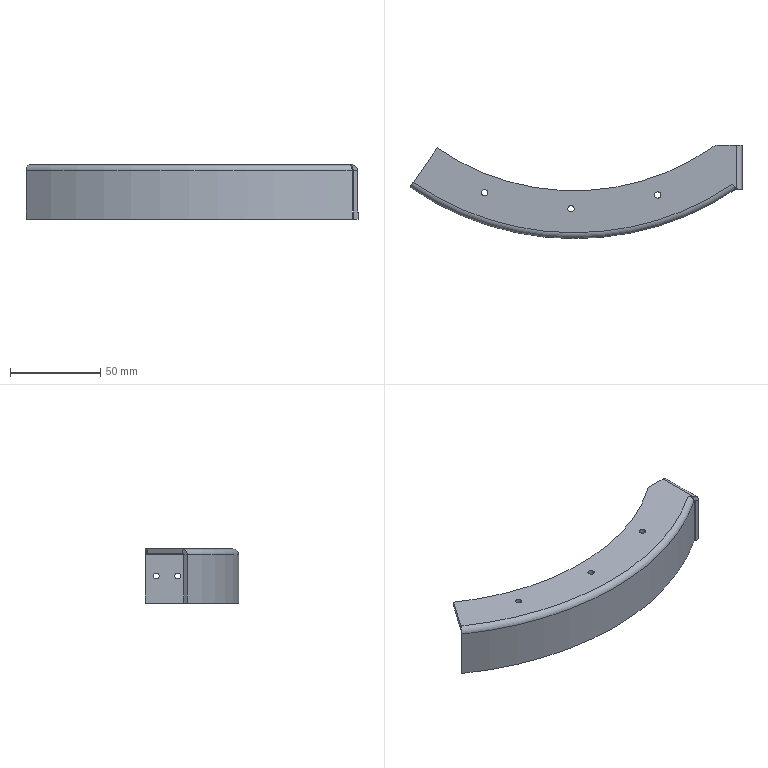Part | SolidWorks | features EdgeFlange 2, 3DProfileFeature 1, Cut 1, Fillet 1, FlatPattern 1, HoleWzd 1, ICE 1, SMBaseFlange 1, SheetMetal 1 | 1 solid | 35 faces | box 184.199 x 51.718 x 30 mm | volume 26604 mm3 | cylinder 16 | plane 16 | torus 2 | spline 1 | commonest cylinder face diameters 3.5 x6 3.3 x4 1.473 x1 6.473 x1 10 x1 267 x1
STEP:
#1=CARTESIAN_POINT('',(90.553,-126.282,-13.35));
#2=VERTEX_POINT('',#1);
#3=CARTESIAN_POINT('',(90.553,-126.282,-16.65));
#4=VERTEX_POINT('',#3);
#5=CARTESIAN_POINT('',(90.553,-126.282,-15.));
#6=DIRECTION('',(1.,0.,0.));
#7=DIRECTION('',(0.,0.,-1.));
#8=AXIS2_PLACEMENT_3D('',#5,#6,#7);
#9=CIRCLE('',#8,1.65);
#10=EDGE_CURVE('',#2,#4,#9,.T.);
#11=ORIENTED_EDGE('',*,*,#10,.F.);
#12=CARTESIAN_POINT('',(93.053,-126.282,-13.35));
#13=VERTEX_POINT('',#12);
#14=CARTESIAN_POINT('',(93.053,-126.282,-13.35));
#15=DIRECTION('',(1.,0.,0.));
#16=VECTOR('',#15,1000.);
#17=LINE('',#14,#16);
#18=EDGE_CURVE('',#2,#13,#17,.T.);
#19=ORIENTED_EDGE('',*,*,#18,.T.);
#20=CARTESIAN_POINT('',(93.053,-126.282,-16.65));
#21=VERTEX_POINT('',#20);
#22=CARTESIAN_POINT('',(93.053,-126.282,-15.));
#23=DIRECTION('',(1.,0.,0.));
#24=DIRECTION('',(0.,0.,-1.));
#25=AXIS2_PLACEMENT_3D('',#22,#23,#24);
#26=CIRCLE('',#25,1.65);
#27=EDGE_CURVE('',#13,#21,#26,.T.);
#28=ORIENTED_EDGE('',*,*,#27,.T.);
#29=CARTESIAN_POINT('',(93.053,-126.282,-16.65));
#30=DIRECTION('',(1.,0.,0.));
#31=VECTOR('',#30,1000.);
#32=LINE('',#29,#31);
#33=EDGE_CURVE('',#4,#21,#32,.T.);
#34=ORIENTED_EDGE('',*,*,#33,.F.);
#35=EDGE_LOOP('',(#11,#19,#28,#34));
#36=FACE_OUTER_BOUND('',#35,.T.);
#37=CARTESIAN_POINT('',(93.053,-126.282,-15.));
#38=DIRECTION('',(1.,0.,0.));
#39=DIRECTION('',(0.,0.,-1.));
#40=AXIS2_PLACEMENT_3D('',#37,#38,#39);
#41=CYLINDRICAL_SURFACE('',#40,1.65);
#42=ADVANCED_FACE('',(#36),#41,.F.);
#43=CARTESIAN_POINT('',(90.553,-114.282,-13.35));
#44=VERTEX_POINT('',#43);
#45=CARTESIAN_POINT('',(90.553,-114.282,-16.65));
#46=VERTEX_POINT('',#45);
#47=CARTESIAN_POINT('',(90.553,-114.282,-15.));
#48=DIRECTION('',(1.,0.,0.));
#49=DIRECTION('',(0.,0.,-1.));
#50=AXIS2_PLACEMENT_3D('',#47,#48,#49);
#51=CIRCLE('',#50,1.65);
#52=EDGE_CURVE('',#44,#46,#51,.T.);
#53=ORIENTED_EDGE('',*,*,#52,.F.);
#54=CARTESIAN_POINT('',(93.053,-114.282,-13.35));
#55=VERTEX_POINT('',#54);
#56=CARTESIAN_POINT('',(93.053,-114.282,-13.35));
#57=DIRECTION('',(1.,0.,0.));
#58=VECTOR('',#57,1000.);
#59=LINE('',#56,#58);
#60=EDGE_CURVE('',#44,#55,#59,.T.);
#61=ORIENTED_EDGE('',*,*,#60,.T.);
#62=CARTESIAN_POINT('',(93.053,-114.282,-16.65));
#63=VERTEX_POINT('',#62);
#64=CARTESIAN_POINT('',(93.053,-114.282,-15.));
#65=DIRECTION('',(1.,0.,0.));
#66=DIRECTION('',(0.,0.,-1.));
#67=AXIS2_PLACEMENT_3D('',#64,#65,#66);
#68=CIRCLE('',#67,1.65);
#69=EDGE_CURVE('',#55,#63,#68,.T.);
#70=ORIENTED_EDGE('',*,*,#69,.T.);
#71=CARTESIAN_POINT('',(93.053,-114.282,-16.65));
#72=DIRECTION('',(1.,0.,0.));
#73=VECTOR('',#72,1000.);
#74=LINE('',#71,#73);
#75=EDGE_CURVE('',#46,#63,#74,.T.);
#76=ORIENTED_EDGE('',*,*,#75,.F.);
#77=EDGE_LOOP('',(#53,#61,#70,#76));
#78=FACE_OUTER_BOUND('',#77,.T.);
#79=CARTESIAN_POINT('',(93.053,-114.282,-15.));
#80=DIRECTION('',(1.,0.,0.));
#81=DIRECTION('',(0.,0.,-1.));
#82=AXIS2_PLACEMENT_3D('',#79,#80,#81);
#83=CYLINDRICAL_SURFACE('',#82,1.65);
#84=ADVANCED_FACE('',(#78),#83,.F.);
#85=CARTESIAN_POINT('',(-3.57,-143.488,-2.5));
#86=VERTEX_POINT('',#85);
#87=CARTESIAN_POINT('',(-0.07006,-143.488,-2.5));
#88=VERTEX_POINT('',#87);
#89=CARTESIAN_POINT('',(-1.82,-143.488,-2.5));
#90=DIRECTION('',(0.,0.,1.));
#91=DIRECTION('',(1.,0.,0.));
#92=AXIS2_PLACEMENT_3D('',#89,#90,#91);
#93=CIRCLE('',#92,1.75);
#94=EDGE_CURVE('',#86,#88,#93,.T.);
#95=ORIENTED_EDGE('',*,*,#94,.F.);
#96=CARTESIAN_POINT('',(-3.57,-143.488,0.));
#97=VERTEX_POINT('',#96);
#98=CARTESIAN_POINT('',(-3.57,-143.488,-30.));
#99=DIRECTION('',(0.,0.,1.));
#100=VECTOR('',#99,1000.);
#101=LINE('',#98,#100);
#102=EDGE_CURVE('',#86,#97,#101,.T.);
#103=ORIENTED_EDGE('',*,*,#102,.T.);
#104=CARTESIAN_POINT('',(-0.07006,-143.488,0.));
#105=VERTEX_POINT('',#104);
#106=CARTESIAN_POINT('',(-1.82,-143.488,0.));
#107=DIRECTION('',(0.,0.,1.));
#108=DIRECTION('',(1.,0.,0.));
#109=AXIS2_PLACEMENT_3D('',#106,#107,#108);
#110=CIRCLE('',#109,1.75);
#111=EDGE_CURVE('',#97,#105,#110,.T.);
#112=ORIENTED_EDGE('',*,*,#111,.T.);
#113=CARTESIAN_POINT('',(-0.07006,-143.488,-30.));
#114=DIRECTION('',(0.,0.,1.));
#115=VECTOR('',#114,1000.);
#116=LINE('',#113,#115);
#117=EDGE_CURVE('',#88,#105,#116,.T.);
#118=ORIENTED_EDGE('',*,*,#117,.F.);
#119=EDGE_LOOP('',(#95,#103,#112,#118));
#120=FACE_OUTER_BOUND('',#119,.T.);
#121=CARTESIAN_POINT('',(-1.82,-143.488,-30.));
#122=DIRECTION('',(0.,0.,1.));
#123=DIRECTION('',(1.,0.,0.));
#124=AXIS2_PLACEMENT_3D('',#121,#122,#123);
#125=CYLINDRICAL_SURFACE('',#124,1.75);
#126=ADVANCED_FACE('',(#120),#125,.F.);
#127=CARTESIAN_POINT('',(44.55,-135.825,-2.5));
#128=VERTEX_POINT('',#127);
#129=CARTESIAN_POINT('',(48.05,-135.825,-2.5));
#130=VERTEX_POINT('',#129);
#131=CARTESIAN_POINT('',(46.3,-135.825,-2.5));
#132=DIRECTION('',(0.,0.,1.));
#133=DIRECTION('',(1.,0.,0.));
#134=AXIS2_PLACEMENT_3D('',#131,#132,#133);
#135=CIRCLE('',#134,1.75);
#136=EDGE_CURVE('',#128,#130,#135,.T.);
#137=ORIENTED_EDGE('',*,*,#136,.F.);
#138=CARTESIAN_POINT('',(44.55,-135.825,0.));
#139=VERTEX_POINT('',#138);
#140=CARTESIAN_POINT('',(44.55,-135.825,-30.));
#141=DIRECTION('',(0.,0.,1.));
#142=VECTOR('',#141,1000.);
#143=LINE('',#140,#142);
#144=EDGE_CURVE('',#128,#139,#143,.T.);
#145=ORIENTED_EDGE('',*,*,#144,.T.);
#146=CARTESIAN_POINT('',(48.05,-135.825,0.));
#147=VERTEX_POINT('',#146);
#148=CARTESIAN_POINT('',(46.3,-135.825,0.));
#149=DIRECTION('',(0.,0.,1.));
#150=DIRECTION('',(1.,0.,0.));
#151=AXIS2_PLACEMENT_3D('',#148,#149,#150);
#152=CIRCLE('',#151,1.75);
#153=EDGE_CURVE('',#139,#147,#152,.T.);
#154=ORIENTED_EDGE('',*,*,#153,.T.);
#155=CARTESIAN_POINT('',(48.05,-135.825,-30.));
#156=DIRECTION('',(0.,0.,1.));
#157=VECTOR('',#156,1000.);
#158=LINE('',#155,#157);
#159=EDGE_CURVE('',#130,#147,#158,.T.);
#160=ORIENTED_EDGE('',*,*,#159,.F.);
#161=EDGE_LOOP('',(#137,#145,#154,#160));
#162=FACE_OUTER_BOUND('',#161,.T.);
#163=CARTESIAN_POINT('',(46.3,-135.825,-30.));
#164=DIRECTION('',(0.,0.,1.));
#165=DIRECTION('',(1.,0.,0.));
#166=AXIS2_PLACEMENT_3D('',#163,#164,#165);
#167=CYLINDRICAL_SURFACE('',#166,1.75);
#168=ADVANCED_FACE('',(#162),#167,.F.);
#169=CARTESIAN_POINT('',(-51.481,-134.607,-2.5));
#170=VERTEX_POINT('',#169);
#171=CARTESIAN_POINT('',(-47.981,-134.607,-2.5));
#172=VERTEX_POINT('',#171);
#173=CARTESIAN_POINT('',(-49.731,-134.607,-2.5));
#174=DIRECTION('',(0.,0.,1.));
#175=DIRECTION('',(1.,0.,0.));
#176=AXIS2_PLACEMENT_3D('',#173,#174,#175);
#177=CIRCLE('',#176,1.75);
#178=EDGE_CURVE('',#170,#172,#177,.T.);
#179=ORIENTED_EDGE('',*,*,#178,.F.);
#180=CARTESIAN_POINT('',(-51.481,-134.607,0.));
#181=VERTEX_POINT('',#180);
#182=CARTESIAN_POINT('',(-51.481,-134.607,-30.));
#183=DIRECTION('',(0.,0.,1.));
#184=VECTOR('',#183,1000.);
#185=LINE('',#182,#184);
#186=EDGE_CURVE('',#170,#181,#185,.T.);
#187=ORIENTED_EDGE('',*,*,#186,.T.);
#188=CARTESIAN_POINT('',(-47.981,-134.607,0.));
#189=VERTEX_POINT('',#188);
#190=CARTESIAN_POINT('',(-49.731,-134.607,0.));
#191=DIRECTION('',(0.,0.,1.));
#192=DIRECTION('',(1.,0.,0.));
#193=AXIS2_PLACEMENT_3D('',#190,#191,#192);
#194=CIRCLE('',#193,1.75);
#195=EDGE_CURVE('',#181,#189,#194,.T.);
#196=ORIENTED_EDGE('',*,*,#195,.T.);
#197=CARTESIAN_POINT('',(-47.981,-134.607,-30.));
#198=DIRECTION('',(0.,0.,1.));
#199=VECTOR('',#198,1000.);
#200=LINE('',#197,#199);
#201=EDGE_CURVE('',#172,#189,#200,.T.);
#202=ORIENTED_EDGE('',*,*,#201,.F.);
#203=EDGE_LOOP('',(#179,#187,#196,#202));
#204=FACE_OUTER_BOUND('',#203,.T.);
#205=CARTESIAN_POINT('',(-49.731,-134.607,-30.));
#206=DIRECTION('',(0.,0.,1.));
#207=DIRECTION('',(1.,0.,0.));
#208=AXIS2_PLACEMENT_3D('',#205,#206,#207);
#209=CYLINDRICAL_SURFACE('',#208,1.75);
#210=ADVANCED_FACE('',(#204),#209,.F.);
#211=CARTESIAN_POINT('',(88.,-129.734,0.));
#212=VERTEX_POINT('',#211);
#213=CARTESIAN_POINT('',(89.816,-132.412,0.));
#214=VERTEX_POINT('',#213);
#215=CARTESIAN_POINT('',(0.,0.,0.));
#216=DIRECTION('',(0.5614,-0.8276,0.));
#217=VECTOR('',#216,1000.);
#218=LINE('',#215,#217);
#219=EDGE_CURVE('',#212,#214,#218,.T.);
#220=ORIENTED_EDGE('',*,*,#219,.F.);
#221=CARTESIAN_POINT('',(89.769,-132.342,-2.5));
#222=VERTEX_POINT('',#221);
#223=CARTESIAN_POINT('',(88.,-129.734,-3.237));
#224=DIRECTION('',(0.8276,0.5614,0.));
#225=DIRECTION('',(0.5614,-0.8276,0.));
#226=AXIS2_PLACEMENT_3D('',#223,#224,#225);
#227=CIRCLE('',#226,3.237);
#228=EDGE_CURVE('',#212,#222,#227,.T.);
#229=ORIENTED_EDGE('',*,*,#228,.T.);
#230=CARTESIAN_POINT('',(89.816,-132.412,-2.5));
#231=VERTEX_POINT('',#230);
#232=CARTESIAN_POINT('',(88.,-129.734,-2.5));
#233=DIRECTION('',(0.5614,-0.8276,0.));
#234=VECTOR('',#233,1000.);
#235=LINE('',#232,#234);
#236=EDGE_CURVE('',#222,#231,#235,.T.);
#237=ORIENTED_EDGE('',*,*,#236,.T.);
#238=CARTESIAN_POINT('',(89.816,-132.412,-2.5));
#239=DIRECTION('',(0.,0.,1.));
#240=VECTOR('',#239,1000.);
#241=LINE('',#238,#240);
#242=EDGE_CURVE('',#231,#214,#241,.T.);
#243=ORIENTED_EDGE('',*,*,#242,.T.);
#244=EDGE_LOOP('',(#220,#229,#237,#243));
#245=FACE_OUTER_BOUND('',#244,.T.);
#246=CARTESIAN_POINT('',(88.,-129.734,-2.5));
#247=DIRECTION('',(-0.8276,-0.5614,0.));
#248=DIRECTION('',(0.5614,-0.8276,0.));
#249=AXIS2_PLACEMENT_3D('',#246,#247,#248);
#250=PLANE('',#249);
#251=ADVANCED_FACE('',(#245),#250,.T.);
#252=CARTESIAN_POINT('',(-1.82,-143.488,-2.5));
#253=DIRECTION('',(0.,0.,1.));
#254=DIRECTION('',(1.,0.,0.));
#255=AXIS2_PLACEMENT_3D('',#252,#253,#254);
#256=CIRCLE('',#255,1.75);
#257=EDGE_CURVE('',#88,#86,#256,.T.);
#258=ORIENTED_EDGE('',*,*,#257,.T.);
#259=ORIENTED_EDGE('',*,*,#94,.T.);
#260=EDGE_LOOP('',(#258,#259));
#261=FACE_BOUND('',#260,.T.);
#262=CARTESIAN_POINT('',(46.3,-135.825,-2.5));
#263=DIRECTION('',(0.,0.,1.));
#264=DIRECTION('',(1.,0.,0.));
#265=AXIS2_PLACEMENT_3D('',#262,#263,#264);
#266=CIRCLE('',#265,1.75);
#267=EDGE_CURVE('',#130,#128,#266,.T.);
#268=ORIENTED_EDGE('',*,*,#267,.T.);
#269=ORIENTED_EDGE('',*,*,#136,.T.);
#270=EDGE_LOOP('',(#268,#269));
#271=FACE_BOUND('',#270,.T.);
#272=CARTESIAN_POINT('',(-49.731,-134.607,-2.5));
#273=DIRECTION('',(0.,0.,1.));
#274=DIRECTION('',(1.,0.,0.));
#275=AXIS2_PLACEMENT_3D('',#272,#273,#274);
#276=CIRCLE('',#275,1.75);
#277=EDGE_CURVE('',#172,#170,#276,.T.);
#278=ORIENTED_EDGE('',*,*,#277,.T.);
#279=ORIENTED_EDGE('',*,*,#178,.T.);
#280=EDGE_LOOP('',(#278,#279));
#281=FACE_BOUND('',#280,.T.);
#282=CARTESIAN_POINT('',(-89.302,-128.84,-2.5));
#283=VERTEX_POINT('',#282);
#284=CARTESIAN_POINT('',(88.,-129.734,-2.5));
#285=VERTEX_POINT('',#284);
#286=CARTESIAN_POINT('',(0.,0.,-2.5));
#287=DIRECTION('',(0.,0.,1.));
#288=DIRECTION('',(-0.5697,-0.8219,0.));
#289=AXIS2_PLACEMENT_3D('',#286,#287,#288);
#290=CIRCLE('',#289,156.763);
#291=EDGE_CURVE('',#283,#285,#290,.T.);
#292=ORIENTED_EDGE('',*,*,#291,.F.);
#293=CARTESIAN_POINT('',(-76.05,-109.721,-2.5));
#294=VERTEX_POINT('',#293);
#295=CARTESIAN_POINT('',(-76.05,-109.721,-2.5));
#296=DIRECTION('',(-0.5697,-0.8219,0.));
#297=VECTOR('',#296,1000.);
#298=LINE('',#295,#297);
#299=EDGE_CURVE('',#294,#283,#298,.T.);
#300=ORIENTED_EDGE('',*,*,#299,.F.);
#301=CARTESIAN_POINT('',(76.05,-109.721,-2.5));
#302=VERTEX_POINT('',#301);
#303=CARTESIAN_POINT('',(0.,0.,-2.5));
#304=DIRECTION('',(0.,0.,-1.));
#305=DIRECTION('',(1.,0.,0.));
#306=AXIS2_PLACEMENT_3D('',#303,#304,#305);
#307=CIRCLE('',#306,133.5);
#308=EDGE_CURVE('',#302,#294,#307,.T.);
#309=ORIENTED_EDGE('',*,*,#308,.F.);
#310=CARTESIAN_POINT('',(79.559,-108.282,-2.5));
#311=VERTEX_POINT('',#310);
#312=CARTESIAN_POINT('',(79.559,-113.282,-2.5));
#313=DIRECTION('',(0.,0.,-1.));
#314=DIRECTION('',(1.,0.,0.));
#315=AXIS2_PLACEMENT_3D('',#312,#313,#314);
#316=CIRCLE('',#315,5.);
#317=EDGE_CURVE('',#302,#311,#316,.T.);
#318=ORIENTED_EDGE('',*,*,#317,.T.);
#319=CARTESIAN_POINT('',(89.816,-108.282,-2.5));
#320=VERTEX_POINT('',#319);
#321=CARTESIAN_POINT('',(75.053,-108.282,-2.5));
#322=DIRECTION('',(1.,0.,0.));
#323=VECTOR('',#322,1000.);
#324=LINE('',#321,#323);
#325=EDGE_CURVE('',#311,#320,#324,.T.);
#326=ORIENTED_EDGE('',*,*,#325,.T.);
#327=CARTESIAN_POINT('',(89.816,-132.939,-2.5));
#328=DIRECTION('',(0.,1.,0.));
#329=VECTOR('',#328,1000.);
#330=LINE('',#327,#329);
#331=EDGE_CURVE('',#231,#320,#330,.T.);
#332=ORIENTED_EDGE('',*,*,#331,.F.);
#333=ORIENTED_EDGE('',*,*,#236,.F.);
#334=CARTESIAN_POINT('',(88.,-129.734,-2.5));
#335=DIRECTION('',(0.5614,-0.8276,0.));
#336=VECTOR('',#335,1000.);
#337=LINE('',#334,#336);
#338=EDGE_CURVE('',#285,#222,#337,.T.);
#339=ORIENTED_EDGE('',*,*,#338,.F.);
#340=EDGE_LOOP('',(#292,#300,#309,#318,#326,#332,#333,#339));
#341=FACE_OUTER_BOUND('',#340,.T.);
#342=CARTESIAN_POINT('',(0.,0.,-2.5));
#343=DIRECTION('',(0.,0.,1.));
#344=DIRECTION('',(1.,0.,0.));
#345=AXIS2_PLACEMENT_3D('',#342,#343,#344);
#346=PLANE('',#345);
#347=ADVANCED_FACE('',(#261,#271,#281,#341),#346,.F.);
#348=CARTESIAN_POINT('',(-1.82,-143.488,0.));
#349=DIRECTION('',(0.,0.,1.));
#350=DIRECTION('',(1.,0.,0.));
#351=AXIS2_PLACEMENT_3D('',#348,#349,#350);
#352=CIRCLE('',#351,1.75);
#353=EDGE_CURVE('',#105,#97,#352,.T.);
#354=ORIENTED_EDGE('',*,*,#353,.F.);
#355=ORIENTED_EDGE('',*,*,#111,.F.);
#356=EDGE_LOOP('',(#354,#355));
#357=FACE_BOUND('',#356,.T.);
#358=CARTESIAN_POINT('',(46.3,-135.825,0.));
#359=DIRECTION('',(0.,0.,1.));
#360=DIRECTION('',(1.,0.,0.));
#361=AXIS2_PLACEMENT_3D('',#358,#359,#360);
#362=CIRCLE('',#361,1.75);
#363=EDGE_CURVE('',#147,#139,#362,.T.);
#364=ORIENTED_EDGE('',*,*,#363,.F.);
#365=ORIENTED_EDGE('',*,*,#153,.F.);
#366=EDGE_LOOP('',(#364,#365));
#367=FACE_BOUND('',#366,.T.);
#368=CARTESIAN_POINT('',(-49.731,-134.607,0.));
#369=DIRECTION('',(0.,0.,1.));
#370=DIRECTION('',(1.,0.,0.));
#371=AXIS2_PLACEMENT_3D('',#368,#369,#370);
#372=CIRCLE('',#371,1.75);
#373=EDGE_CURVE('',#189,#181,#372,.T.);
#374=ORIENTED_EDGE('',*,*,#373,.F.);
#375=ORIENTED_EDGE('',*,*,#195,.F.);
#376=EDGE_LOOP('',(#374,#375));
#377=FACE_BOUND('',#376,.T.);
#378=CARTESIAN_POINT('',(-76.05,-109.721,0.));
#379=VERTEX_POINT('',#378);
#380=CARTESIAN_POINT('',(-89.302,-128.84,0.));
#381=VERTEX_POINT('',#380);
#382=CARTESIAN_POINT('',(-76.05,-109.721,0.));
#383=DIRECTION('',(-0.5697,-0.8219,0.));
#384=VECTOR('',#383,1000.);
#385=LINE('',#382,#384);
#386=EDGE_CURVE('',#379,#381,#385,.T.);
#387=ORIENTED_EDGE('',*,*,#386,.T.);
#388=CARTESIAN_POINT('',(0.,0.,0.));
#389=DIRECTION('',(0.,0.,1.));
#390=DIRECTION('',(1.,0.,0.));
#391=AXIS2_PLACEMENT_3D('',#388,#389,#390);
#392=CIRCLE('',#391,156.763);
#393=EDGE_CURVE('',#381,#212,#392,.T.);
#394=ORIENTED_EDGE('',*,*,#393,.T.);
#395=ORIENTED_EDGE('',*,*,#219,.T.);
#396=CARTESIAN_POINT('',(89.816,-108.282,0.));
#397=VERTEX_POINT('',#396);
#398=CARTESIAN_POINT('',(89.816,-132.939,0.));
#399=DIRECTION('',(0.,1.,0.));
#400=VECTOR('',#399,1000.);
#401=LINE('',#398,#400);
#402=EDGE_CURVE('',#214,#397,#401,.T.);
#403=ORIENTED_EDGE('',*,*,#402,.T.);
#404=CARTESIAN_POINT('',(79.559,-108.282,0.));
#405=VERTEX_POINT('',#404);
#406=CARTESIAN_POINT('',(75.053,-108.282,0.));
#407=DIRECTION('',(-1.,0.,0.));
#408=VECTOR('',#407,1000.);
#409=LINE('',#406,#408);
#410=EDGE_CURVE('',#397,#405,#409,.T.);
#411=ORIENTED_EDGE('',*,*,#410,.T.);
#412=CARTESIAN_POINT('',(76.05,-109.721,0.));
#413=VERTEX_POINT('',#412);
#414=CARTESIAN_POINT('',(79.559,-113.282,0.));
#415=DIRECTION('',(0.,0.,1.));
#416=DIRECTION('',(1.,0.,0.));
#417=AXIS2_PLACEMENT_3D('',#414,#415,#416);
#418=CIRCLE('',#417,5.);
#419=EDGE_CURVE('',#405,#413,#418,.T.);
#420=ORIENTED_EDGE('',*,*,#419,.T.);
#421=CARTESIAN_POINT('',(0.,0.,0.));
#422=DIRECTION('',(0.,0.,-1.));
#423=DIRECTION('',(1.,0.,0.));
#424=AXIS2_PLACEMENT_3D('',#421,#422,#423);
#425=CIRCLE('',#424,133.5);
#426=EDGE_CURVE('',#413,#379,#425,.T.);
#427=ORIENTED_EDGE('',*,*,#426,.T.);
#428=EDGE_LOOP('',(#387,#394,#395,#403,#411,#420,#427));
#429=FACE_OUTER_BOUND('',#428,.T.);
#430=CARTESIAN_POINT('',(0.,0.,0.));
#431=DIRECTION('',(0.,0.,1.));
#432=DIRECTION('',(1.,0.,0.));
#433=AXIS2_PLACEMENT_3D('',#430,#431,#432);
#434=PLANE('',#433);
#435=ADVANCED_FACE('',(#357,#367,#377,#429),#434,.T.);
#436=CARTESIAN_POINT('',(-89.302,-128.84,-2.5));
#437=DIRECTION('',(0.,0.,1.));
#438=VECTOR('',#437,1000.);
#439=LINE('',#436,#438);
#440=EDGE_CURVE('',#283,#381,#439,.T.);
#441=ORIENTED_EDGE('',*,*,#440,.T.);
#442=ORIENTED_EDGE('',*,*,#386,.F.);
#443=CARTESIAN_POINT('',(-76.05,-109.721,-2.5));
#444=DIRECTION('',(0.,0.,1.));
#445=VECTOR('',#444,1000.);
#446=LINE('',#443,#445);
#447=EDGE_CURVE('',#294,#379,#446,.T.);
#448=ORIENTED_EDGE('',*,*,#447,.F.);
#449=ORIENTED_EDGE('',*,*,#299,.T.);
#450=EDGE_LOOP('',(#441,#442,#448,#449));
#451=FACE_OUTER_BOUND('',#450,.T.);
#452=CARTESIAN_POINT('',(-76.05,-109.721,-2.5));
#453=DIRECTION('',(-0.8219,0.5697,0.));
#454=DIRECTION('',(-0.5697,-0.8219,0.));
#455=AXIS2_PLACEMENT_3D('',#452,#453,#454);
#456=PLANE('',#455);
#457=ADVANCED_FACE('',(#451),#456,.T.);
#458=ORIENTED_EDGE('',*,*,#426,.F.);
#459=CARTESIAN_POINT('',(76.05,-109.721,-2.5));
#460=DIRECTION('',(0.,0.,1.));
#461=VECTOR('',#460,1000.);
#462=LINE('',#459,#461);
#463=EDGE_CURVE('',#302,#413,#462,.T.);
#464=ORIENTED_EDGE('',*,*,#463,.F.);
#465=ORIENTED_EDGE('',*,*,#308,.T.);
#466=ORIENTED_EDGE('',*,*,#447,.T.);
#467=EDGE_LOOP('',(#458,#464,#465,#466));
#468=FACE_OUTER_BOUND('',#467,.T.);
#469=CARTESIAN_POINT('',(0.,0.,-2.5));
#470=DIRECTION('',(0.,0.,1.));
#471=DIRECTION('',(1.,0.,0.));
#472=AXIS2_PLACEMENT_3D('',#469,#470,#471);
#473=CYLINDRICAL_SURFACE('',#472,133.5);
#474=ADVANCED_FACE('',(#468),#473,.F.);
#475=ORIENTED_EDGE('',*,*,#325,.F.);
#476=CARTESIAN_POINT('',(79.559,-108.282,0.));
#477=DIRECTION('',(0.,0.,1.));
#478=VECTOR('',#477,1000.);
#479=LINE('',#476,#478);
#480=EDGE_CURVE('',#311,#405,#479,.T.);
#481=ORIENTED_EDGE('',*,*,#480,.T.);
#482=ORIENTED_EDGE('',*,*,#410,.F.);
#483=CARTESIAN_POINT('',(89.816,-108.282,-2.5));
#484=DIRECTION('',(0.,0.,1.));
#485=VECTOR('',#484,1000.);
#486=LINE('',#483,#485);
#487=EDGE_CURVE('',#320,#397,#486,.T.);
#488=ORIENTED_EDGE('',*,*,#487,.F.);
#489=EDGE_LOOP('',(#475,#481,#482,#488));
#490=FACE_OUTER_BOUND('',#489,.T.);
#491=CARTESIAN_POINT('',(75.053,-108.282,-33.028));
#492=DIRECTION('',(0.,1.,0.));
#493=DIRECTION('',(-1.,0.,0.));
#494=AXIS2_PLACEMENT_3D('',#491,#492,#493);
#495=PLANE('',#494);
#496=ADVANCED_FACE('',(#490),#495,.T.);
#497=CARTESIAN_POINT('',(90.553,-108.282,-3.237));
#498=VERTEX_POINT('',#497);
#499=CARTESIAN_POINT('',(93.053,-108.282,-3.237));
#500=VERTEX_POINT('',#499);
#501=CARTESIAN_POINT('',(93.053,-108.282,-3.237));
#502=DIRECTION('',(1.,0.,0.));
#503=VECTOR('',#502,1000.);
#504=LINE('',#501,#503);
#505=EDGE_CURVE('',#498,#500,#504,.T.);
#506=ORIENTED_EDGE('',*,*,#505,.F.);
#507=CARTESIAN_POINT('',(89.816,-108.282,-3.237));
#508=DIRECTION('',(0.,1.,0.));
#509=DIRECTION('',(0.,0.,-1.));
#510=AXIS2_PLACEMENT_3D('',#507,#508,#509);
#511=CIRCLE('',#510,0.7366);
#512=EDGE_CURVE('',#320,#498,#511,.T.);
#513=ORIENTED_EDGE('',*,*,#512,.F.);
#514=ORIENTED_EDGE('',*,*,#487,.T.);
#515=CARTESIAN_POINT('',(89.816,-108.282,-3.237));
#516=DIRECTION('',(0.,1.,0.));
#517=DIRECTION('',(0.,0.,-1.));
#518=AXIS2_PLACEMENT_3D('',#515,#516,#517);
#519=CIRCLE('',#518,3.237);
#520=EDGE_CURVE('',#397,#500,#519,.T.);
#521=ORIENTED_EDGE('',*,*,#520,.T.);
#522=EDGE_LOOP('',(#506,#513,#514,#521));
#523=FACE_OUTER_BOUND('',#522,.T.);
#524=CARTESIAN_POINT('',(89.816,-108.282,-3.237));
#525=DIRECTION('',(0.,1.,0.));
#526=DIRECTION('',(0.,0.,1.));
#527=AXIS2_PLACEMENT_3D('',#524,#525,#526);
#528=PLANE('',#527);
#529=ADVANCED_FACE('',(#523),#528,.T.);
#530=CARTESIAN_POINT('',(90.553,-132.939,-3.237));
#531=VERTEX_POINT('',#530);
#532=CARTESIAN_POINT('',(90.553,-132.939,-3.237));
#533=CARTESIAN_POINT('',(90.553,-132.851,-3.044));
#534=CARTESIAN_POINT('',(90.474,-132.763,-2.852));
#535=CARTESIAN_POINT('',(90.201,-132.588,-2.579));
#536=CARTESIAN_POINT('',(90.009,-132.5,-2.5));
#537=CARTESIAN_POINT('',(89.816,-132.412,-2.5));
#538=B_SPLINE_CURVE_WITH_KNOTS('',3,(#532,#533,#534,#535,#536,#537),.UNSPECIFIED.,.F.,.F.,(4,2,4),(0.,0.5,1.),.UNSPECIFIED.);
#539=EDGE_CURVE('',#531,#231,#538,.T.);
#540=ORIENTED_EDGE('',*,*,#539,.F.);
#541=CARTESIAN_POINT('',(93.053,-132.939,-3.237));
#542=VERTEX_POINT('',#541);
#543=CARTESIAN_POINT('',(90.553,-132.939,-3.237));
#544=DIRECTION('',(1.,0.,0.));
#545=VECTOR('',#544,1000.);
#546=LINE('',#543,#545);
#547=EDGE_CURVE('',#531,#542,#546,.T.);
#548=ORIENTED_EDGE('',*,*,#547,.T.);
#549=CARTESIAN_POINT('',(93.053,-132.939,-3.237));
#550=CARTESIAN_POINT('',(93.053,-132.895,-2.813));
#551=CARTESIAN_POINT('',(92.969,-132.851,-2.389));
#552=CARTESIAN_POINT('',(92.645,-132.763,-1.607));
#553=CARTESIAN_POINT('',(92.405,-132.719,-1.248));
#554=CARTESIAN_POINT('',(91.806,-132.632,-0.6484));
#555=CARTESIAN_POINT('',(91.447,-132.588,-0.4085));
#556=CARTESIAN_POINT('',(90.664,-132.5,-0.08424));
#557=CARTESIAN_POINT('',(90.24,-132.456,0.));
#558=CARTESIAN_POINT('',(89.816,-132.412,0.));
#559=B_SPLINE_CURVE_WITH_KNOTS('',3,(#549,#550,#551,#552,#553,#554,#555,#556,#557,#558),.UNSPECIFIED.,.F.,.F.,(4,2,2,2,4),(0.,0.25,0.5,0.75,1.),.UNSPECIFIED.);
#560=EDGE_CURVE('',#542,#214,#559,.T.);
#561=ORIENTED_EDGE('',*,*,#560,.T.);
#562=ORIENTED_EDGE('',*,*,#242,.F.);
#563=EDGE_LOOP('',(#540,#548,#561,#562));
#564=FACE_OUTER_BOUND('',#563,.T.);
#565=CARTESIAN_POINT('',(93.078,-132.939,-3.237));
#566=CARTESIAN_POINT('',(93.078,-132.895,-2.81));
#567=CARTESIAN_POINT('',(92.993,-132.851,-2.383));
#568=CARTESIAN_POINT('',(92.666,-132.763,-1.594));
#569=CARTESIAN_POINT('',(92.425,-132.719,-1.232));
#570=CARTESIAN_POINT('',(91.821,-132.632,-0.6284));
#571=CARTESIAN_POINT('',(91.459,-132.588,-0.3867));
#572=CARTESIAN_POINT('',(90.67,-132.5,-0.05989));
#573=CARTESIAN_POINT('',(90.244,-132.456,0.025));
#574=CARTESIAN_POINT('',(89.816,-132.412,0.025));
#575=CARTESIAN_POINT('',(93.053,-132.939,-3.237));
#576=CARTESIAN_POINT('',(93.053,-132.895,-2.813));
#577=CARTESIAN_POINT('',(92.969,-132.851,-2.389));
#578=CARTESIAN_POINT('',(92.645,-132.763,-1.607));
#579=CARTESIAN_POINT('',(92.405,-132.719,-1.248));
#580=CARTESIAN_POINT('',(91.806,-132.632,-0.6484));
#581=CARTESIAN_POINT('',(91.447,-132.588,-0.4085));
#582=CARTESIAN_POINT('',(90.664,-132.5,-0.08424));
#583=CARTESIAN_POINT('',(90.24,-132.456,0.));
#584=CARTESIAN_POINT('',(89.816,-132.412,0.));
#585=CARTESIAN_POINT('',(90.553,-132.939,-3.237));
#586=CARTESIAN_POINT('',(90.553,-132.895,-3.14));
#587=CARTESIAN_POINT('',(90.534,-132.851,-3.044));
#588=CARTESIAN_POINT('',(90.46,-132.763,-2.866));
#589=CARTESIAN_POINT('',(90.406,-132.719,-2.784));
#590=CARTESIAN_POINT('',(90.269,-132.632,-2.648));
#591=CARTESIAN_POINT('',(90.187,-132.588,-2.593));
#592=CARTESIAN_POINT('',(90.009,-132.5,-2.519));
#593=CARTESIAN_POINT('',(89.913,-132.456,-2.5));
#594=CARTESIAN_POINT('',(89.816,-132.412,-2.5));
#595=CARTESIAN_POINT('',(90.528,-132.939,-3.237));
#596=CARTESIAN_POINT('',(90.528,-132.895,-3.143));
#597=CARTESIAN_POINT('',(90.509,-132.851,-3.05));
#598=CARTESIAN_POINT('',(90.438,-132.763,-2.878));
#599=CARTESIAN_POINT('',(90.385,-132.719,-2.799));
#600=CARTESIAN_POINT('',(90.254,-132.632,-2.668));
#601=CARTESIAN_POINT('',(90.175,-132.588,-2.615));
#602=CARTESIAN_POINT('',(90.003,-132.5,-2.544));
#603=CARTESIAN_POINT('',(89.91,-132.456,-2.525));
#604=CARTESIAN_POINT('',(89.816,-132.412,-2.525));
#605=B_SPLINE_SURFACE_WITH_KNOTS('',1,3,((#565,#566,#567,#568,#569,#570,#571,#572,#573,#574),(#575,#576,#577,#578,#579,#580,#581,#582,#583,#584),(#585,#586,#587,#588,#589,#590,#591,#592,#593,#594),(#595,#596,#597,#598,#599,#600,#601,#602,#603,#604)),.UNSPECIFIED.,.F.,.F.,.F.,(2,1,1,2),(4,2,2,2,4),(-0.01,0.,1.,1.01),(0.,0.25,0.5,0.75,1.),.UNSPECIFIED.);
#606=ADVANCED_FACE('',(#564),#605,.F.);
#607=ORIENTED_EDGE('',*,*,#402,.F.);
#608=ORIENTED_EDGE('',*,*,#560,.F.);
#609=CARTESIAN_POINT('',(93.053,0.,-3.237));
#610=DIRECTION('',(0.,-1.,0.));
#611=VECTOR('',#610,1000.);
#612=LINE('',#609,#611);
#613=EDGE_CURVE('',#500,#542,#612,.T.);
#614=ORIENTED_EDGE('',*,*,#613,.F.);
#615=ORIENTED_EDGE('',*,*,#520,.F.);
#616=EDGE_LOOP('',(#607,#608,#614,#615));
#617=FACE_OUTER_BOUND('',#616,.T.);
#618=CARTESIAN_POINT('',(89.816,-132.939,-3.237));
#619=DIRECTION('',(0.,-1.,0.));
#620=DIRECTION('',(1.,0.,0.));
#621=AXIS2_PLACEMENT_3D('',#618,#619,#620);
#622=CYLINDRICAL_SURFACE('',#621,3.237);
#623=ADVANCED_FACE('',(#617),#622,.T.);
#624=ORIENTED_EDGE('',*,*,#331,.T.);
#625=ORIENTED_EDGE('',*,*,#512,.T.);
#626=CARTESIAN_POINT('',(90.553,-108.282,-3.237));
#627=DIRECTION('',(0.,-1.,0.));
#628=VECTOR('',#627,1000.);
#629=LINE('',#626,#628);
#630=EDGE_CURVE('',#498,#531,#629,.T.);
#631=ORIENTED_EDGE('',*,*,#630,.T.);
#632=ORIENTED_EDGE('',*,*,#539,.T.);
#633=EDGE_LOOP('',(#624,#625,#631,#632));
#634=FACE_OUTER_BOUND('',#633,.T.);
#635=CARTESIAN_POINT('',(89.816,-132.939,-3.237));
#636=DIRECTION('',(0.,-1.,0.));
#637=DIRECTION('',(1.,0.,0.));
#638=AXIS2_PLACEMENT_3D('',#635,#636,#637);
#639=CYLINDRICAL_SURFACE('',#638,0.7366);
#640=ADVANCED_FACE('',(#634),#639,.F.);
#641=CARTESIAN_POINT('',(93.053,-132.939,-30.));
#642=VERTEX_POINT('',#641);
#643=CARTESIAN_POINT('',(93.053,-132.939,-2.5));
#644=DIRECTION('',(0.,0.,1.));
#645=VECTOR('',#644,1000.);
#646=LINE('',#643,#645);
#647=EDGE_CURVE('',#642,#542,#646,.T.);
#648=ORIENTED_EDGE('',*,*,#647,.T.);
#649=ORIENTED_EDGE('',*,*,#547,.F.);
#650=CARTESIAN_POINT('',(90.553,-132.939,-30.));
#651=VERTEX_POINT('',#650);
#652=CARTESIAN_POINT('',(90.553,-132.939,0.));
#653=DIRECTION('',(0.,0.,1.));
#654=VECTOR('',#653,1000.);
#655=LINE('',#652,#654);
#656=EDGE_CURVE('',#651,#531,#655,.T.);
#657=ORIENTED_EDGE('',*,*,#656,.F.);
#658=CARTESIAN_POINT('',(93.053,-132.939,-30.));
#659=DIRECTION('',(-1.,0.,0.));
#660=VECTOR('',#659,1000.);
#661=LINE('',#658,#660);
#662=EDGE_CURVE('',#642,#651,#661,.T.);
#663=ORIENTED_EDGE('',*,*,#662,.F.);
#664=EDGE_LOOP('',(#648,#649,#657,#663));
#665=FACE_OUTER_BOUND('',#664,.T.);
#666=CARTESIAN_POINT('',(93.053,-132.939,-2.5));
#667=DIRECTION('',(0.,-1.,0.));
#668=DIRECTION('',(0.,0.,-1.));
#669=AXIS2_PLACEMENT_3D('',#666,#667,#668);
#670=PLANE('',#669);
#671=ADVANCED_FACE('',(#665),#670,.T.);
#672=CARTESIAN_POINT('',(90.553,-108.282,-30.));
#673=VERTEX_POINT('',#672);
#674=CARTESIAN_POINT('',(90.553,-108.282,0.));
#675=DIRECTION('',(0.,0.,-1.));
#676=VECTOR('',#675,1000.);
#677=LINE('',#674,#676);
#678=EDGE_CURVE('',#498,#673,#677,.T.);
#679=ORIENTED_EDGE('',*,*,#678,.F.);
#680=ORIENTED_EDGE('',*,*,#505,.T.);
#681=CARTESIAN_POINT('',(93.053,-108.282,-30.));
#682=VERTEX_POINT('',#681);
#683=CARTESIAN_POINT('',(93.053,-108.282,-30.));
#684=DIRECTION('',(0.,0.,-1.));
#685=VECTOR('',#684,1000.);
#686=LINE('',#683,#685);
#687=EDGE_CURVE('',#500,#682,#686,.T.);
#688=ORIENTED_EDGE('',*,*,#687,.T.);
#689=CARTESIAN_POINT('',(93.053,-108.282,-30.));
#690=DIRECTION('',(-1.,0.,0.));
#691=VECTOR('',#690,1000.);
#692=LINE('',#689,#691);
#693=EDGE_CURVE('',#682,#673,#692,.T.);
#694=ORIENTED_EDGE('',*,*,#693,.T.);
#695=EDGE_LOOP('',(#679,#680,#688,#694));
#696=FACE_OUTER_BOUND('',#695,.T.);
#697=CARTESIAN_POINT('',(93.053,-108.282,-30.));
#698=DIRECTION('',(0.,1.,0.));
#699=DIRECTION('',(0.,0.,1.));
#700=AXIS2_PLACEMENT_3D('',#697,#698,#699);
#701=PLANE('',#700);
#702=ADVANCED_FACE('',(#696),#701,.T.);
#703=CARTESIAN_POINT('',(93.053,-126.282,-15.));
#704=DIRECTION('',(1.,0.,0.));
#705=DIRECTION('',(0.,0.,-1.));
#706=AXIS2_PLACEMENT_3D('',#703,#704,#705);
#707=CIRCLE('',#706,1.65);
#708=EDGE_CURVE('',#21,#13,#707,.T.);
#709=ORIENTED_EDGE('',*,*,#708,.F.);
#710=ORIENTED_EDGE('',*,*,#27,.F.);
#711=EDGE_LOOP('',(#709,#710));
#712=FACE_BOUND('',#711,.T.);
#713=CARTESIAN_POINT('',(93.053,-114.282,-15.));
#714=DIRECTION('',(1.,0.,0.));
#715=DIRECTION('',(0.,0.,-1.));
#716=AXIS2_PLACEMENT_3D('',#713,#714,#715);
#717=CIRCLE('',#716,1.65);
#718=EDGE_CURVE('',#63,#55,#717,.T.);
#719=ORIENTED_EDGE('',*,*,#718,.F.);
#720=ORIENTED_EDGE('',*,*,#69,.F.);
#721=EDGE_LOOP('',(#719,#720));
#722=FACE_BOUND('',#721,.T.);
#723=ORIENTED_EDGE('',*,*,#687,.F.);
#724=ORIENTED_EDGE('',*,*,#613,.T.);
#725=ORIENTED_EDGE('',*,*,#647,.F.);
#726=CARTESIAN_POINT('',(93.053,-132.939,-30.));
#727=DIRECTION('',(0.,-1.,0.));
#728=VECTOR('',#727,1000.);
#729=LINE('',#726,#728);
#730=EDGE_CURVE('',#682,#642,#729,.T.);
#731=ORIENTED_EDGE('',*,*,#730,.F.);
#732=EDGE_LOOP('',(#723,#724,#725,#731));
#733=FACE_OUTER_BOUND('',#732,.T.);
#734=CARTESIAN_POINT('',(93.053,0.,0.));
#735=DIRECTION('',(1.,0.,0.));
#736=DIRECTION('',(0.,0.,-1.));
#737=AXIS2_PLACEMENT_3D('',#734,#735,#736);
#738=PLANE('',#737);
#739=ADVANCED_FACE('',(#712,#722,#733),#738,.T.);
#740=CARTESIAN_POINT('',(90.553,-126.282,-15.));
#741=DIRECTION('',(1.,0.,0.));
#742=DIRECTION('',(0.,0.,-1.));
#743=AXIS2_PLACEMENT_3D('',#740,#741,#742);
#744=CIRCLE('',#743,1.65);
#745=EDGE_CURVE('',#4,#2,#744,.T.);
#746=ORIENTED_EDGE('',*,*,#745,.T.);
#747=ORIENTED_EDGE('',*,*,#10,.T.);
#748=EDGE_LOOP('',(#746,#747));
#749=FACE_BOUND('',#748,.T.);
#750=CARTESIAN_POINT('',(90.553,-114.282,-15.));
#751=DIRECTION('',(1.,0.,0.));
#752=DIRECTION('',(0.,0.,-1.));
#753=AXIS2_PLACEMENT_3D('',#750,#751,#752);
#754=CIRCLE('',#753,1.65);
#755=EDGE_CURVE('',#46,#44,#754,.T.);
#756=ORIENTED_EDGE('',*,*,#755,.T.);
#757=ORIENTED_EDGE('',*,*,#52,.T.);
#758=EDGE_LOOP('',(#756,#757));
#759=FACE_BOUND('',#758,.T.);
#760=ORIENTED_EDGE('',*,*,#630,.F.);
#761=ORIENTED_EDGE('',*,*,#678,.T.);
#762=CARTESIAN_POINT('',(90.553,0.,-30.));
#763=DIRECTION('',(0.,-1.,0.));
#764=VECTOR('',#763,1000.);
#765=LINE('',#762,#764);
#766=EDGE_CURVE('',#673,#651,#765,.T.);
#767=ORIENTED_EDGE('',*,*,#766,.T.);
#768=ORIENTED_EDGE('',*,*,#656,.T.);
#769=EDGE_LOOP('',(#760,#761,#767,#768));
#770=FACE_OUTER_BOUND('',#769,.T.);
#771=CARTESIAN_POINT('',(90.553,0.,0.));
#772=DIRECTION('',(1.,0.,0.));
#773=DIRECTION('',(0.,0.,-1.));
#774=AXIS2_PLACEMENT_3D('',#771,#772,#773);
#775=PLANE('',#774);
#776=ADVANCED_FACE('',(#749,#759,#770),#775,.F.);
#777=ORIENTED_EDGE('',*,*,#766,.F.);
#778=ORIENTED_EDGE('',*,*,#693,.F.);
#779=ORIENTED_EDGE('',*,*,#730,.T.);
#780=ORIENTED_EDGE('',*,*,#662,.T.);
#781=EDGE_LOOP('',(#777,#778,#779,#780));
#782=FACE_OUTER_BOUND('',#781,.T.);
#783=CARTESIAN_POINT('',(93.053,-132.939,-30.));
#784=DIRECTION('',(0.,0.,-1.));
#785=DIRECTION('',(-1.,0.,0.));
#786=AXIS2_PLACEMENT_3D('',#783,#784,#785);
#787=PLANE('',#786);
#788=ADVANCED_FACE('',(#782),#787,.T.);
#789=ORIENTED_EDGE('',*,*,#317,.F.);
#790=ORIENTED_EDGE('',*,*,#463,.T.);
#791=ORIENTED_EDGE('',*,*,#419,.F.);
#792=ORIENTED_EDGE('',*,*,#480,.F.);
#793=EDGE_LOOP('',(#789,#790,#791,#792));
#794=FACE_OUTER_BOUND('',#793,.T.);
#795=CARTESIAN_POINT('',(79.559,-113.282,-2.5));
#796=DIRECTION('',(0.,0.,1.));
#797=DIRECTION('',(1.,0.,0.));
#798=AXIS2_PLACEMENT_3D('',#795,#796,#797);
#799=CYLINDRICAL_SURFACE('',#798,5.);
#800=ADVANCED_FACE('',(#794),#799,.T.);
#801=CARTESIAN_POINT('',(88.413,-130.343,-3.237));
#802=VERTEX_POINT('',#801);
#803=CARTESIAN_POINT('',(88.,-129.734,-3.237));
#804=DIRECTION('',(0.8276,0.5614,0.));
#805=DIRECTION('',(0.5614,-0.8276,0.));
#806=AXIS2_PLACEMENT_3D('',#803,#804,#805);
#807=CIRCLE('',#806,0.7366);
#808=EDGE_CURVE('',#285,#802,#807,.T.);
#809=ORIENTED_EDGE('',*,*,#808,.F.);
#810=ORIENTED_EDGE('',*,*,#338,.T.);
#811=CARTESIAN_POINT('',(89.816,-132.412,-3.237));
#812=VERTEX_POINT('',#811);
#813=CARTESIAN_POINT('',(88.,-129.734,-3.237));
#814=DIRECTION('',(0.8276,0.5614,0.));
#815=DIRECTION('',(0.5614,-0.8276,0.));
#816=AXIS2_PLACEMENT_3D('',#813,#814,#815);
#817=CIRCLE('',#816,3.237);
#818=EDGE_CURVE('',#222,#812,#817,.T.);
#819=ORIENTED_EDGE('',*,*,#818,.T.);
#820=CARTESIAN_POINT('',(88.413,-130.343,-3.237));
#821=DIRECTION('',(0.5614,-0.8276,0.));
#822=VECTOR('',#821,1000.);
#823=LINE('',#820,#822);
#824=EDGE_CURVE('',#802,#812,#823,.T.);
#825=ORIENTED_EDGE('',*,*,#824,.F.);
#826=EDGE_LOOP('',(#809,#810,#819,#825));
#827=FACE_OUTER_BOUND('',#826,.T.);
#828=CARTESIAN_POINT('',(88.,-129.734,-3.237));
#829=DIRECTION('',(0.8276,0.5614,0.));
#830=DIRECTION('',(-0.5614,0.8276,0.));
#831=AXIS2_PLACEMENT_3D('',#828,#829,#830);
#832=PLANE('',#831);
#833=ADVANCED_FACE('',(#827),#832,.T.);
#834=ORIENTED_EDGE('',*,*,#440,.F.);
#835=CARTESIAN_POINT('',(-89.722,-129.446,-3.237));
#836=VERTEX_POINT('',#835);
#837=CARTESIAN_POINT('',(-89.302,-128.84,-3.237));
#838=DIRECTION('',(0.8219,-0.5697,0.));
#839=DIRECTION('',(-0.5697,-0.8219,0.));
#840=AXIS2_PLACEMENT_3D('',#837,#838,#839);
#841=CIRCLE('',#840,0.7366);
#842=EDGE_CURVE('',#283,#836,#841,.T.);
#843=ORIENTED_EDGE('',*,*,#842,.T.);
#844=CARTESIAN_POINT('',(-91.146,-131.501,-3.237));
#845=VERTEX_POINT('',#844);
#846=CARTESIAN_POINT('',(-89.722,-129.446,-3.237));
#847=DIRECTION('',(-0.5697,-0.8219,0.));
#848=VECTOR('',#847,1000.);
#849=LINE('',#846,#848);
#850=EDGE_CURVE('',#836,#845,#849,.T.);
#851=ORIENTED_EDGE('',*,*,#850,.T.);
#852=CARTESIAN_POINT('',(-89.302,-128.84,-3.237));
#853=DIRECTION('',(0.8219,-0.5697,0.));
#854=DIRECTION('',(-0.5697,-0.8219,0.));
#855=AXIS2_PLACEMENT_3D('',#852,#853,#854);
#856=CIRCLE('',#855,3.237);
#857=EDGE_CURVE('',#381,#845,#856,.T.);
#858=ORIENTED_EDGE('',*,*,#857,.F.);
#859=EDGE_LOOP('',(#834,#843,#851,#858));
#860=FACE_OUTER_BOUND('',#859,.T.);
#861=CARTESIAN_POINT('',(-89.302,-128.84,-3.237));
#862=DIRECTION('',(0.8219,-0.5697,0.));
#863=DIRECTION('',(0.5697,0.8219,0.));
#864=AXIS2_PLACEMENT_3D('',#861,#862,#863);
#865=PLANE('',#864);
#866=ADVANCED_FACE('',(#860),#865,.F.);
#867=ORIENTED_EDGE('',*,*,#850,.F.);
#868=CARTESIAN_POINT('',(-89.722,-129.446,-30.));
#869=VERTEX_POINT('',#868);
#870=CARTESIAN_POINT('',(-89.722,-129.446,-2.5));
#871=DIRECTION('',(0.,0.,-1.));
#872=VECTOR('',#871,1000.);
#873=LINE('',#870,#872);
#874=EDGE_CURVE('',#836,#869,#873,.T.);
#875=ORIENTED_EDGE('',*,*,#874,.T.);
#876=CARTESIAN_POINT('',(-91.146,-131.501,-30.));
#877=VERTEX_POINT('',#876);
#878=CARTESIAN_POINT('',(-89.722,-129.446,-30.));
#879=DIRECTION('',(-0.5697,-0.8219,0.));
#880=VECTOR('',#879,1000.);
#881=LINE('',#878,#880);
#882=EDGE_CURVE('',#869,#877,#881,.T.);
#883=ORIENTED_EDGE('',*,*,#882,.T.);
#884=CARTESIAN_POINT('',(-91.146,-131.501,-2.5));
#885=DIRECTION('',(0.,0.,-1.));
#886=VECTOR('',#885,1000.);
#887=LINE('',#884,#886);
#888=EDGE_CURVE('',#845,#877,#887,.T.);
#889=ORIENTED_EDGE('',*,*,#888,.F.);
#890=EDGE_LOOP('',(#867,#875,#883,#889));
#891=FACE_OUTER_BOUND('',#890,.T.);
#892=CARTESIAN_POINT('',(-89.722,-129.446,-16.618));
#893=DIRECTION('',(-0.8219,0.5697,0.));
#894=DIRECTION('',(0.,0.,-1.));
#895=AXIS2_PLACEMENT_3D('',#892,#893,#894);
#896=PLANE('',#895);
#897=ADVANCED_FACE('',(#891),#896,.T.);
#898=ORIENTED_EDGE('',*,*,#882,.F.);
#899=CARTESIAN_POINT('',(88.413,-130.343,-30.));
#900=VERTEX_POINT('',#899);
#901=CARTESIAN_POINT('',(0.,0.,-30.));
#902=DIRECTION('',(0.,0.,1.));
#903=DIRECTION('',(-0.5697,-0.8219,0.));
#904=AXIS2_PLACEMENT_3D('',#901,#902,#903);
#905=CIRCLE('',#904,157.5);
#906=EDGE_CURVE('',#869,#900,#905,.T.);
#907=ORIENTED_EDGE('',*,*,#906,.T.);
#908=CARTESIAN_POINT('',(89.816,-132.412,-30.));
#909=VERTEX_POINT('',#908);
#910=CARTESIAN_POINT('',(88.413,-130.343,-30.));
#911=DIRECTION('',(0.5614,-0.8276,0.));
#912=VECTOR('',#911,1000.);
#913=LINE('',#910,#912);
#914=EDGE_CURVE('',#900,#909,#913,.T.);
#915=ORIENTED_EDGE('',*,*,#914,.T.);
#916=CARTESIAN_POINT('',(0.,0.,-30.));
#917=DIRECTION('',(0.,0.,1.));
#918=DIRECTION('',(1.,0.,0.));
#919=AXIS2_PLACEMENT_3D('',#916,#917,#918);
#920=CIRCLE('',#919,160.);
#921=EDGE_CURVE('',#877,#909,#920,.T.);
#922=ORIENTED_EDGE('',*,*,#921,.F.);
#923=EDGE_LOOP('',(#898,#907,#915,#922));
#924=FACE_OUTER_BOUND('',#923,.T.);
#925=CARTESIAN_POINT('',(0.,0.,-30.));
#926=DIRECTION('',(0.,0.,-1.));
#927=DIRECTION('',(-1.,0.,0.));
#928=AXIS2_PLACEMENT_3D('',#925,#926,#927);
#929=PLANE('',#928);
#930=ADVANCED_FACE('',(#924),#929,.T.);
#931=CARTESIAN_POINT('',(88.413,-130.343,-2.5));
#932=DIRECTION('',(0.,0.,-1.));
#933=VECTOR('',#932,1000.);
#934=LINE('',#931,#933);
#935=EDGE_CURVE('',#802,#900,#934,.T.);
#936=ORIENTED_EDGE('',*,*,#935,.F.);
#937=ORIENTED_EDGE('',*,*,#824,.T.);
#938=CARTESIAN_POINT('',(89.816,-132.412,-2.5));
#939=DIRECTION('',(0.,0.,-1.));
#940=VECTOR('',#939,1000.);
#941=LINE('',#938,#940);
#942=EDGE_CURVE('',#812,#909,#941,.T.);
#943=ORIENTED_EDGE('',*,*,#942,.T.);
#944=ORIENTED_EDGE('',*,*,#914,.F.);
#945=EDGE_LOOP('',(#936,#937,#943,#944));
#946=FACE_OUTER_BOUND('',#945,.T.);
#947=CARTESIAN_POINT('',(88.413,-130.343,-16.618));
#948=DIRECTION('',(-0.8276,-0.5614,0.));
#949=DIRECTION('',(0.,0.,-1.));
#950=AXIS2_PLACEMENT_3D('',#947,#948,#949);
#951=PLANE('',#950);
#952=ADVANCED_FACE('',(#946),#951,.F.);
#953=ORIENTED_EDGE('',*,*,#921,.T.);
#954=ORIENTED_EDGE('',*,*,#942,.F.);
#955=CARTESIAN_POINT('',(0.,0.,-3.237));
#956=DIRECTION('',(0.,0.,1.));
#957=DIRECTION('',(1.,0.,0.));
#958=AXIS2_PLACEMENT_3D('',#955,#956,#957);
#959=CIRCLE('',#958,160.);
#960=EDGE_CURVE('',#845,#812,#959,.T.);
#961=ORIENTED_EDGE('',*,*,#960,.F.);
#962=ORIENTED_EDGE('',*,*,#888,.T.);
#963=EDGE_LOOP('',(#953,#954,#961,#962));
#964=FACE_OUTER_BOUND('',#963,.T.);
#965=CARTESIAN_POINT('',(0.,0.,-2.5));
#966=DIRECTION('',(0.,0.,1.));
#967=DIRECTION('',(1.,0.,0.));
#968=AXIS2_PLACEMENT_3D('',#965,#966,#967);
#969=CYLINDRICAL_SURFACE('',#968,160.);
#970=ADVANCED_FACE('',(#964),#969,.T.);
#971=ORIENTED_EDGE('',*,*,#960,.T.);
#972=ORIENTED_EDGE('',*,*,#818,.F.);
#973=ORIENTED_EDGE('',*,*,#228,.F.);
#974=ORIENTED_EDGE('',*,*,#393,.F.);
#975=ORIENTED_EDGE('',*,*,#857,.T.);
#976=EDGE_LOOP('',(#971,#972,#973,#974,#975));
#977=FACE_OUTER_BOUND('',#976,.T.);
#978=CARTESIAN_POINT('',(0.,0.,-3.237));
#979=DIRECTION('',(0.,0.,1.));
#980=DIRECTION('',(1.,0.,0.));
#981=AXIS2_PLACEMENT_3D('',#978,#979,#980);
#982=TOROIDAL_SURFACE('',#981,156.763,3.237);
#983=ADVANCED_FACE('',(#977),#982,.T.);
#984=ORIENTED_EDGE('',*,*,#906,.F.);
#985=ORIENTED_EDGE('',*,*,#874,.F.);
#986=CARTESIAN_POINT('',(0.,0.,-3.237));
#987=DIRECTION('',(0.,0.,1.));
#988=DIRECTION('',(-0.5697,-0.8219,0.));
#989=AXIS2_PLACEMENT_3D('',#986,#987,#988);
#990=CIRCLE('',#989,157.5);
#991=EDGE_CURVE('',#836,#802,#990,.T.);
#992=ORIENTED_EDGE('',*,*,#991,.T.);
#993=ORIENTED_EDGE('',*,*,#935,.T.);
#994=EDGE_LOOP('',(#984,#985,#992,#993));
#995=FACE_OUTER_BOUND('',#994,.T.);
#996=CARTESIAN_POINT('',(0.,0.,-2.5));
#997=DIRECTION('',(0.,0.,1.));
#998=DIRECTION('',(1.,0.,0.));
#999=AXIS2_PLACEMENT_3D('',#996,#997,#998);
#1000=CYLINDRICAL_SURFACE('',#999,157.5);
#1001=ADVANCED_FACE('',(#995),#1000,.F.);
#1002=ORIENTED_EDGE('',*,*,#991,.F.);
#1003=ORIENTED_EDGE('',*,*,#842,.F.);
#1004=ORIENTED_EDGE('',*,*,#291,.T.);
#1005=ORIENTED_EDGE('',*,*,#808,.T.);
#1006=EDGE_LOOP('',(#1002,#1003,#1004,#1005));
#1007=FACE_OUTER_BOUND('',#1006,.T.);
#1008=CARTESIAN_POINT('',(0.,0.,-3.237));
#1009=DIRECTION('',(0.,0.,1.));
#1010=DIRECTION('',(1.,0.,0.));
#1011=AXIS2_PLACEMENT_3D('',#1008,#1009,#1010);
#1012=TOROIDAL_SURFACE('',#1011,156.763,0.7366);
#1013=ADVANCED_FACE('',(#1007),#1012,.F.);
#1014=ORIENTED_EDGE('',*,*,#186,.F.);
#1015=ORIENTED_EDGE('',*,*,#277,.F.);
#1016=ORIENTED_EDGE('',*,*,#201,.T.);
#1017=ORIENTED_EDGE('',*,*,#373,.T.);
#1018=EDGE_LOOP('',(#1014,#1015,#1016,#1017));
#1019=FACE_OUTER_BOUND('',#1018,.T.);
#1020=CARTESIAN_POINT('',(-49.731,-134.607,-30.));
#1021=DIRECTION('',(0.,0.,1.));
#1022=DIRECTION('',(1.,0.,0.));
#1023=AXIS2_PLACEMENT_3D('',#1020,#1021,#1022);
#1024=CYLINDRICAL_SURFACE('',#1023,1.75);
#1025=ADVANCED_FACE('',(#1019),#1024,.F.);
#1026=ORIENTED_EDGE('',*,*,#144,.F.);
#1027=ORIENTED_EDGE('',*,*,#267,.F.);
#1028=ORIENTED_EDGE('',*,*,#159,.T.);
#1029=ORIENTED_EDGE('',*,*,#363,.T.);
#1030=EDGE_LOOP('',(#1026,#1027,#1028,#1029));
#1031=FACE_OUTER_BOUND('',#1030,.T.);
#1032=CARTESIAN_POINT('',(46.3,-135.825,-30.));
#1033=DIRECTION('',(0.,0.,1.));
#1034=DIRECTION('',(1.,0.,0.));
#1035=AXIS2_PLACEMENT_3D('',#1032,#1033,#1034);
#1036=CYLINDRICAL_SURFACE('',#1035,1.75);
#1037=ADVANCED_FACE('',(#1031),#1036,.F.);
#1038=ORIENTED_EDGE('',*,*,#102,.F.);
#1039=ORIENTED_EDGE('',*,*,#257,.F.);
#1040=ORIENTED_EDGE('',*,*,#117,.T.);
#1041=ORIENTED_EDGE('',*,*,#353,.T.);
#1042=EDGE_LOOP('',(#1038,#1039,#1040,#1041));
#1043=FACE_OUTER_BOUND('',#1042,.T.);
#1044=CARTESIAN_POINT('',(-1.82,-143.488,-30.));
#1045=DIRECTION('',(0.,0.,1.));
#1046=DIRECTION('',(1.,0.,0.));
#1047=AXIS2_PLACEMENT_3D('',#1044,#1045,#1046);
#1048=CYLINDRICAL_SURFACE('',#1047,1.75);
#1049=ADVANCED_FACE('',(#1043),#1048,.F.);
#1050=ORIENTED_EDGE('',*,*,#60,.F.);
#1051=ORIENTED_EDGE('',*,*,#755,.F.);
#1052=ORIENTED_EDGE('',*,*,#75,.T.);
#1053=ORIENTED_EDGE('',*,*,#718,.T.);
#1054=EDGE_LOOP('',(#1050,#1051,#1052,#1053));
#1055=FACE_OUTER_BOUND('',#1054,.T.);
#1056=CARTESIAN_POINT('',(93.053,-114.282,-15.));
#1057=DIRECTION('',(1.,0.,0.));
#1058=DIRECTION('',(0.,0.,-1.));
#1059=AXIS2_PLACEMENT_3D('',#1056,#1057,#1058);
#1060=CYLINDRICAL_SURFACE('',#1059,1.65);
#1061=ADVANCED_FACE('',(#1055),#1060,.F.);
#1062=ORIENTED_EDGE('',*,*,#18,.F.);
#1063=ORIENTED_EDGE('',*,*,#745,.F.);
#1064=ORIENTED_EDGE('',*,*,#33,.T.);
#1065=ORIENTED_EDGE('',*,*,#708,.T.);
#1066=EDGE_LOOP('',(#1062,#1063,#1064,#1065));
#1067=FACE_OUTER_BOUND('',#1066,.T.);
#1068=CARTESIAN_POINT('',(93.053,-126.282,-15.));
#1069=DIRECTION('',(1.,0.,0.));
#1070=DIRECTION('',(0.,0.,-1.));
#1071=AXIS2_PLACEMENT_3D('',#1068,#1069,#1070);
#1072=CYLINDRICAL_SURFACE('',#1071,1.65);
#1073=ADVANCED_FACE('',(#1067),#1072,.F.);
#1074=CLOSED_SHELL('',(#42,#84,#126,#168,#210,#251,#347,#435,#457,#474,#496,#529,#606,#623,#640,#671,#702,#739,#776,#788,#800,#833,#866,#897,#930,#952,#970,#983,#1001,#1013,#1025,#1037,#1049,#1061,#1073));
#1075=MANIFOLD_SOLID_BREP('',#1074);
#1076=CARTESIAN_POINT('',(0.,0.,0.));
#1077=DIRECTION('',(0.,0.,1.));
#1078=DIRECTION('',(1.,0.,0.));
#1079=AXIS2_PLACEMENT_3D('',#1076,#1077,#1078);
#1080=(LENGTH_UNIT()NAMED_UNIT(*)SI_UNIT(.MILLI.,.METRE.));
#1081=UNCERTAINTY_MEASURE_WITH_UNIT(LENGTH_MEASURE(0.00001),#1080,'','');
#1082=(NAMED_UNIT(*)PLANE_ANGLE_UNIT()SI_UNIT($,.RADIAN.));
#1083=(NAMED_UNIT(*)SI_UNIT($,.STERADIAN.)SOLID_ANGLE_UNIT());
#1084=(GEOMETRIC_REPRESENTATION_CONTEXT(3)GLOBAL_UNCERTAINTY_ASSIGNED_CONTEXT((#1081))GLOBAL_UNIT_ASSIGNED_CONTEXT((#1080,#1082,#1083))REPRESENTATION_CONTEXT('',''));
#1085=ADVANCED_BREP_SHAPE_REPRESENTATION('',(#1075,#1079),#1084);